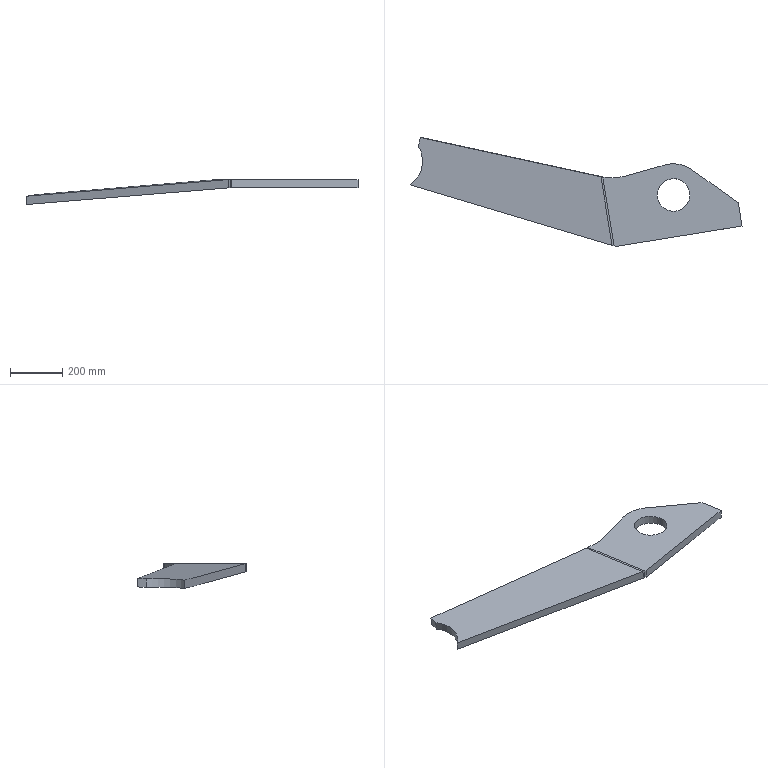Part | SolidWorks | features SplitBody 1 | 1 solid | 22 faces | box 1274 x 418.793 x 95.912 mm | volume 8572989 mm3 | plane 12 | cylinder 8 | spline 2 | commonest cylinder face diameters 125 x2 400 x2 100 x1 164 x1 220 x1 240 x1
STEP:
#1=CARTESIAN_POINT('',(4252.633,293.982,-770.5));
#2=VERTEX_POINT('',#1);
#3=CARTESIAN_POINT('',(4129.247,273.958,-770.5));
#4=VERTEX_POINT('',#3);
#5=CARTESIAN_POINT('',(4190.94,283.97,-770.5));
#6=DIRECTION('',(0.,0.,-1.));
#7=DIRECTION('',(-0.9871,-0.1602,0.));
#8=AXIS2_PLACEMENT_3D('',#5,#6,#7);
#9=CIRCLE('',#8,62.5);
#10=EDGE_CURVE('',#2,#4,#9,.T.);
#11=ORIENTED_EDGE('',*,*,#10,.F.);
#12=CARTESIAN_POINT('',(4252.633,293.982,-802.5));
#13=VERTEX_POINT('',#12);
#14=CARTESIAN_POINT('',(4252.633,293.982,-770.5));
#15=DIRECTION('',(0.,0.,-1.));
#16=VECTOR('',#15,1000.);
#17=LINE('',#14,#16);
#18=EDGE_CURVE('',#2,#13,#17,.T.);
#19=ORIENTED_EDGE('',*,*,#18,.T.);
#20=CARTESIAN_POINT('',(4129.247,273.958,-802.5));
#21=VERTEX_POINT('',#20);
#22=CARTESIAN_POINT('',(4190.94,283.97,-802.5));
#23=DIRECTION('',(0.,0.,-1.));
#24=DIRECTION('',(-0.9871,-0.1602,0.));
#25=AXIS2_PLACEMENT_3D('',#22,#23,#24);
#26=CIRCLE('',#25,62.5);
#27=EDGE_CURVE('',#13,#21,#26,.T.);
#28=ORIENTED_EDGE('',*,*,#27,.T.);
#29=CARTESIAN_POINT('',(4129.247,273.958,-770.5));
#30=DIRECTION('',(0.,0.,-1.));
#31=VECTOR('',#30,1000.);
#32=LINE('',#29,#31);
#33=EDGE_CURVE('',#4,#21,#32,.T.);
#34=ORIENTED_EDGE('',*,*,#33,.F.);
#35=EDGE_LOOP('',(#11,#19,#28,#34));
#36=FACE_OUTER_BOUND('',#35,.T.);
#37=CARTESIAN_POINT('',(4190.94,283.97,-770.5));
#38=DIRECTION('',(0.,0.,-1.));
#39=DIRECTION('',(-0.9871,-0.1602,0.));
#40=AXIS2_PLACEMENT_3D('',#37,#38,#39);
#41=CYLINDRICAL_SURFACE('',#40,62.5);
#42=ADVANCED_FACE('',(#36),#41,.F.);
#43=CARTESIAN_POINT('',(3957.472,90.301,-802.69));
#44=VERTEX_POINT('',#43);
#45=CARTESIAN_POINT('',(3914.616,354.364,-802.69));
#46=VERTEX_POINT('',#45);
#47=CARTESIAN_POINT('',(3884.78,538.207,-802.69));
#48=DIRECTION('',(-0.1602,0.9871,0.));
#49=VECTOR('',#48,1000.);
#50=LINE('',#47,#49);
#51=EDGE_CURVE('',#44,#46,#50,.T.);
#52=ORIENTED_EDGE('',*,*,#51,.F.);
#53=CARTESIAN_POINT('',(3181.855,322.901,-866.412));
#54=VERTEX_POINT('',#53);
#55=CARTESIAN_POINT('',(3181.855,322.901,-866.412));
#56=DIRECTION('',(0.9549,-0.2864,0.07845));
#57=VECTOR('',#56,1000.);
#58=LINE('',#55,#57);
#59=EDGE_CURVE('',#54,#44,#58,.T.);
#60=ORIENTED_EDGE('',*,*,#59,.F.);
#61=CARTESIAN_POINT('',(3214.351,471.062,-861.529));
#62=VERTEX_POINT('',#61);
#63=CARTESIAN_POINT('',(3120.615,414.189,-870.421));
#64=DIRECTION('',(0.08603,0.01396,-0.9962));
#65=DIRECTION('',(-0.9833,-0.1596,-0.08716));
#66=AXIS2_PLACEMENT_3D('',#63,#64,#65);
#67=CIRCLE('',#66,110.);
#68=EDGE_CURVE('',#62,#54,#67,.T.);
#69=ORIENTED_EDGE('',*,*,#68,.F.);
#70=CARTESIAN_POINT('',(3221.578,504.78,-860.432));
#71=VERTEX_POINT('',#70);
#72=CARTESIAN_POINT('',(3221.578,504.78,-860.432));
#73=DIRECTION('',(-0.2095,-0.9773,-0.03179));
#74=VECTOR('',#73,1000.);
#75=LINE('',#72,#74);
#76=EDGE_CURVE('',#71,#62,#75,.T.);
#77=ORIENTED_EDGE('',*,*,#76,.F.);
#78=CARTESIAN_POINT('',(3914.552,354.378,-802.696));
#79=VERTEX_POINT('',#78);
#80=CARTESIAN_POINT('',(3914.552,354.378,-802.696));
#81=DIRECTION('',(-0.974,0.2114,-0.08115));
#82=VECTOR('',#81,1000.);
#83=LINE('',#80,#82);
#84=EDGE_CURVE('',#79,#71,#83,.T.);
#85=ORIENTED_EDGE('',*,*,#84,.F.);
#86=CARTESIAN_POINT('',(3956.445,549.838,-796.338));
#87=DIRECTION('',(-0.08603,-0.01396,0.9962));
#88=DIRECTION('',(-0.9833,-0.1596,-0.08716));
#89=AXIS2_PLACEMENT_3D('',#86,#87,#88);
#90=CIRCLE('',#89,200.);
#91=EDGE_CURVE('',#79,#46,#90,.T.);
#92=ORIENTED_EDGE('',*,*,#91,.T.);
#93=EDGE_LOOP('',(#52,#60,#69,#77,#85,#92));
#94=FACE_OUTER_BOUND('',#93,.T.);
#95=CARTESIAN_POINT('',(3120.615,414.189,-870.421));
#96=DIRECTION('',(-0.08603,-0.01396,0.9962));
#97=DIRECTION('',(0.9833,0.1596,0.08716));
#98=AXIS2_PLACEMENT_3D('',#95,#96,#97);
#99=PLANE('',#98);
#100=ADVANCED_FACE('',(#94),#99,.F.);
#101=CARTESIAN_POINT('',(3919.263,352.938,-802.5));
#102=VERTEX_POINT('',#101);
#103=CARTESIAN_POINT('',(3919.263,352.938,-802.5));
#104=CARTESIAN_POINT('',(3917.712,353.413,-802.5));
#105=CARTESIAN_POINT('',(3916.162,353.888,-802.564));
#106=CARTESIAN_POINT('',(3914.616,354.364,-802.69));
#107=B_SPLINE_CURVE_WITH_KNOTS('',3,(#103,#104,#105,#106),.UNSPECIFIED.,.F.,.F.,(4,4),(0.,1.),.UNSPECIFIED.);
#108=EDGE_CURVE('',#102,#46,#107,.T.);
#109=ORIENTED_EDGE('',*,*,#108,.F.);
#110=CARTESIAN_POINT('',(3962.22,88.248,-802.5));
#111=VERTEX_POINT('',#110);
#112=CARTESIAN_POINT('',(3983.96,-45.707,-802.5));
#113=DIRECTION('',(-0.1602,0.9871,0.));
#114=VECTOR('',#113,1000.);
#115=LINE('',#112,#114);
#116=EDGE_CURVE('',#111,#102,#115,.T.);
#117=ORIENTED_EDGE('',*,*,#116,.F.);
#118=CARTESIAN_POINT('',(3957.472,90.301,-802.69));
#119=CARTESIAN_POINT('',(3959.051,89.616,-802.564));
#120=CARTESIAN_POINT('',(3960.635,88.932,-802.5));
#121=CARTESIAN_POINT('',(3962.22,88.248,-802.5));
#122=B_SPLINE_CURVE_WITH_KNOTS('',3,(#118,#119,#120,#121),.UNSPECIFIED.,.F.,.F.,(4,4),(0.,1.),.UNSPECIFIED.);
#123=EDGE_CURVE('',#44,#111,#122,.T.);
#124=ORIENTED_EDGE('',*,*,#123,.F.);
#125=ORIENTED_EDGE('',*,*,#51,.T.);
#126=EDGE_LOOP('',(#109,#117,#124,#125));
#127=FACE_OUTER_BOUND('',#126,.T.);
#128=CARTESIAN_POINT('',(3983.96,-45.707,-852.5));
#129=DIRECTION('',(-0.1602,0.9871,0.));
#130=DIRECTION('',(-0.08603,-0.01396,0.9962));
#131=AXIS2_PLACEMENT_3D('',#128,#129,#130);
#132=CYLINDRICAL_SURFACE('',#131,50.);
#133=ADVANCED_FACE('',(#127),#132,.F.);
#134=CARTESIAN_POINT('',(3954.719,89.855,-770.812));
#135=VERTEX_POINT('',#134);
#136=CARTESIAN_POINT('',(3954.719,89.855,-770.812));
#137=DIRECTION('',(0.08603,0.01396,-0.9962));
#138=VECTOR('',#137,1000.);
#139=LINE('',#136,#138);
#140=EDGE_CURVE('',#135,#44,#139,.T.);
#141=ORIENTED_EDGE('',*,*,#140,.F.);
#142=CARTESIAN_POINT('',(3179.102,322.454,-834.533));
#143=VERTEX_POINT('',#142);
#144=CARTESIAN_POINT('',(3179.102,322.454,-834.533));
#145=DIRECTION('',(0.9549,-0.2864,0.07845));
#146=VECTOR('',#145,1000.);
#147=LINE('',#144,#146);
#148=EDGE_CURVE('',#143,#135,#147,.T.);
#149=ORIENTED_EDGE('',*,*,#148,.F.);
#150=CARTESIAN_POINT('',(3179.102,322.454,-834.533));
#151=DIRECTION('',(-0.08603,-0.01396,0.9962));
#152=VECTOR('',#151,1000.);
#153=LINE('',#150,#152);
#154=EDGE_CURVE('',#54,#143,#153,.T.);
#155=ORIENTED_EDGE('',*,*,#154,.F.);
#156=ORIENTED_EDGE('',*,*,#59,.T.);
#157=EDGE_LOOP('',(#141,#149,#155,#156));
#158=FACE_OUTER_BOUND('',#157,.T.);
#159=CARTESIAN_POINT('',(3179.102,322.454,-834.533));
#160=DIRECTION('',(0.2842,0.958,0.03797));
#161=DIRECTION('',(-0.9549,0.2864,-0.07845));
#162=AXIS2_PLACEMENT_3D('',#159,#160,#161);
#163=PLANE('',#162);
#164=ADVANCED_FACE('',(#158),#163,.F.);
#165=ORIENTED_EDGE('',*,*,#154,.T.);
#166=CARTESIAN_POINT('',(3211.598,470.615,-829.651));
#167=VERTEX_POINT('',#166);
#168=CARTESIAN_POINT('',(3117.862,413.742,-838.543));
#169=DIRECTION('',(0.08603,0.01396,-0.9962));
#170=DIRECTION('',(-0.9833,-0.1596,-0.08716));
#171=AXIS2_PLACEMENT_3D('',#168,#169,#170);
#172=CIRCLE('',#171,110.);
#173=EDGE_CURVE('',#167,#143,#172,.T.);
#174=ORIENTED_EDGE('',*,*,#173,.F.);
#175=CARTESIAN_POINT('',(3211.598,470.615,-829.651));
#176=DIRECTION('',(-0.08603,-0.01396,0.9962));
#177=VECTOR('',#176,1000.);
#178=LINE('',#175,#177);
#179=EDGE_CURVE('',#62,#167,#178,.T.);
#180=ORIENTED_EDGE('',*,*,#179,.F.);
#181=ORIENTED_EDGE('',*,*,#68,.T.);
#182=EDGE_LOOP('',(#165,#174,#180,#181));
#183=FACE_OUTER_BOUND('',#182,.T.);
#184=CARTESIAN_POINT('',(3117.862,413.742,-838.543));
#185=DIRECTION('',(0.08603,0.01396,-0.9962));
#186=DIRECTION('',(-0.9833,-0.1596,-0.08716));
#187=AXIS2_PLACEMENT_3D('',#184,#185,#186);
#188=CYLINDRICAL_SURFACE('',#187,110.);
#189=ADVANCED_FACE('',(#183),#188,.F.);
#190=ORIENTED_EDGE('',*,*,#179,.T.);
#191=CARTESIAN_POINT('',(3218.825,504.333,-828.554));
#192=VERTEX_POINT('',#191);
#193=CARTESIAN_POINT('',(3218.825,504.333,-828.554));
#194=DIRECTION('',(-0.2095,-0.9773,-0.03179));
#195=VECTOR('',#194,1000.);
#196=LINE('',#193,#195);
#197=EDGE_CURVE('',#192,#167,#196,.T.);
#198=ORIENTED_EDGE('',*,*,#197,.F.);
#199=CARTESIAN_POINT('',(3218.825,504.333,-828.554));
#200=DIRECTION('',(-0.08603,-0.01396,0.9962));
#201=VECTOR('',#200,1000.);
#202=LINE('',#199,#201);
#203=EDGE_CURVE('',#71,#192,#202,.T.);
#204=ORIENTED_EDGE('',*,*,#203,.F.);
#205=ORIENTED_EDGE('',*,*,#76,.T.);
#206=EDGE_LOOP('',(#190,#198,#204,#205));
#207=FACE_OUTER_BOUND('',#206,.T.);
#208=CARTESIAN_POINT('',(3218.825,504.333,-828.554));
#209=DIRECTION('',(0.974,-0.2114,0.08115));
#210=DIRECTION('',(0.2095,0.9773,0.03179));
#211=AXIS2_PLACEMENT_3D('',#208,#209,#210);
#212=PLANE('',#211);
#213=ADVANCED_FACE('',(#207),#212,.F.);
#214=ORIENTED_EDGE('',*,*,#203,.T.);
#215=CARTESIAN_POINT('',(3911.799,353.931,-770.817));
#216=VERTEX_POINT('',#215);
#217=CARTESIAN_POINT('',(3218.825,504.333,-828.554));
#218=DIRECTION('',(-0.974,0.2114,-0.08115));
#219=VECTOR('',#218,1000.);
#220=LINE('',#217,#219);
#221=EDGE_CURVE('',#216,#192,#220,.T.);
#222=ORIENTED_EDGE('',*,*,#221,.F.);
#223=CARTESIAN_POINT('',(3911.799,353.931,-770.817));
#224=DIRECTION('',(-0.08603,-0.01396,0.9962));
#225=VECTOR('',#224,1000.);
#226=LINE('',#223,#225);
#227=EDGE_CURVE('',#79,#216,#226,.T.);
#228=ORIENTED_EDGE('',*,*,#227,.F.);
#229=ORIENTED_EDGE('',*,*,#84,.T.);
#230=EDGE_LOOP('',(#214,#222,#228,#229));
#231=FACE_OUTER_BOUND('',#230,.T.);
#232=CARTESIAN_POINT('',(3218.825,504.333,-828.554));
#233=DIRECTION('',(-0.2095,-0.9773,-0.03179));
#234=DIRECTION('',(0.974,-0.2114,0.08115));
#235=AXIS2_PLACEMENT_3D('',#232,#233,#234);
#236=PLANE('',#235);
#237=ADVANCED_FACE('',(#231),#236,.F.);
#238=CARTESIAN_POINT('',(3911.863,353.917,-770.812));
#239=VERTEX_POINT('',#238);
#240=CARTESIAN_POINT('',(3913.24,354.141,-786.751));
#241=DIRECTION('',(-0.08603,-0.01396,0.9962));
#242=VECTOR('',#241,1000.);
#243=LINE('',#240,#242);
#244=EDGE_CURVE('',#46,#239,#243,.T.);
#245=ORIENTED_EDGE('',*,*,#244,.T.);
#246=CARTESIAN_POINT('',(3919.263,352.938,-770.5));
#247=VERTEX_POINT('',#246);
#248=CARTESIAN_POINT('',(3911.863,353.917,-770.812));
#249=CARTESIAN_POINT('',(3914.324,353.59,-770.604));
#250=CARTESIAN_POINT('',(3916.793,353.264,-770.5));
#251=CARTESIAN_POINT('',(3919.263,352.938,-770.5));
#252=B_SPLINE_CURVE_WITH_KNOTS('',3,(#248,#249,#250,#251),.UNSPECIFIED.,.F.,.F.,(4,4),(0.,1.),.UNSPECIFIED.);
#253=EDGE_CURVE('',#239,#247,#252,.T.);
#254=ORIENTED_EDGE('',*,*,#253,.T.);
#255=CARTESIAN_POINT('',(3919.263,352.938,-786.5));
#256=DIRECTION('',(0.,0.,-1.));
#257=VECTOR('',#256,1000.);
#258=LINE('',#255,#257);
#259=EDGE_CURVE('',#247,#102,#258,.T.);
#260=ORIENTED_EDGE('',*,*,#259,.T.);
#261=ORIENTED_EDGE('',*,*,#108,.T.);
#262=EDGE_LOOP('',(#245,#254,#260,#261));
#263=FACE_OUTER_BOUND('',#262,.T.);
#264=CARTESIAN_POINT('',(3919.263,352.938,-770.18));
#265=CARTESIAN_POINT('',(3916.784,353.262,-770.18));
#266=CARTESIAN_POINT('',(3914.306,353.587,-770.285));
#267=CARTESIAN_POINT('',(3911.836,353.913,-770.493));
#268=CARTESIAN_POINT('',(3919.263,352.938,-770.5));
#269=CARTESIAN_POINT('',(3916.793,353.264,-770.5));
#270=CARTESIAN_POINT('',(3914.324,353.59,-770.604));
#271=CARTESIAN_POINT('',(3911.863,353.917,-770.812));
#272=CARTESIAN_POINT('',(3919.263,352.938,-802.5));
#273=CARTESIAN_POINT('',(3917.712,353.413,-802.5));
#274=CARTESIAN_POINT('',(3916.162,353.888,-802.564));
#275=CARTESIAN_POINT('',(3914.616,354.364,-802.69));
#276=B_SPLINE_SURFACE_WITH_KNOTS('',1,3,((#264,#265,#266,#267),(#268,#269,#270,#271),(#272,#273,#274,#275)),.UNSPECIFIED.,.F.,.F.,.F.,(2,1,2),(4,4),(-0.01,0.,1.),(0.,1.),.UNSPECIFIED.);
#277=ADVANCED_FACE('',(#263),#276,.T.);
#278=CARTESIAN_POINT('',(4190.94,283.97,-802.5));
#279=DIRECTION('',(0.,0.,-1.));
#280=DIRECTION('',(-0.9871,-0.1602,0.));
#281=AXIS2_PLACEMENT_3D('',#278,#279,#280);
#282=CIRCLE('',#281,62.5);
#283=EDGE_CURVE('',#21,#13,#282,.T.);
#284=ORIENTED_EDGE('',*,*,#283,.F.);
#285=ORIENTED_EDGE('',*,*,#27,.F.);
#286=EDGE_LOOP('',(#284,#285));
#287=FACE_BOUND('',#286,.T.);
#288=CARTESIAN_POINT('',(4010.04,357.285,-802.5));
#289=VERTEX_POINT('',#288);
#290=CARTESIAN_POINT('',(3955.335,549.658,-802.5));
#291=DIRECTION('',(0.,0.,-1.));
#292=DIRECTION('',(-0.9871,-0.1602,0.));
#293=AXIS2_PLACEMENT_3D('',#290,#291,#292);
#294=CIRCLE('',#293,200.);
#295=EDGE_CURVE('',#289,#102,#294,.T.);
#296=ORIENTED_EDGE('',*,*,#295,.F.);
#297=CARTESIAN_POINT('',(4158.117,399.394,-802.5));
#298=VERTEX_POINT('',#297);
#299=CARTESIAN_POINT('',(4158.117,399.394,-802.5));
#300=DIRECTION('',(-0.9619,-0.2735,0.));
#301=VECTOR('',#300,1000.);
#302=LINE('',#299,#301);
#303=EDGE_CURVE('',#298,#289,#302,.T.);
#304=ORIENTED_EDGE('',*,*,#303,.F.);
#305=CARTESIAN_POINT('',(4261.011,381.386,-802.5));
#306=VERTEX_POINT('',#305);
#307=CARTESIAN_POINT('',(4190.94,283.97,-802.5));
#308=DIRECTION('',(0.,0.,1.));
#309=DIRECTION('',(-0.9871,-0.1602,0.));
#310=AXIS2_PLACEMENT_3D('',#307,#308,#309);
#311=CIRCLE('',#310,120.);
#312=EDGE_CURVE('',#306,#298,#311,.T.);
#313=ORIENTED_EDGE('',*,*,#312,.F.);
#314=CARTESIAN_POINT('',(4439.054,253.321,-802.5));
#315=VERTEX_POINT('',#314);
#316=CARTESIAN_POINT('',(4439.054,253.321,-802.5));
#317=DIRECTION('',(-0.8118,0.5839,0.));
#318=VECTOR('',#317,1000.);
#319=LINE('',#316,#318);
#320=EDGE_CURVE('',#315,#306,#319,.T.);
#321=ORIENTED_EDGE('',*,*,#320,.F.);
#322=CARTESIAN_POINT('',(4453.472,164.483,-802.5));
#323=VERTEX_POINT('',#322);
#324=CARTESIAN_POINT('',(4379.781,618.543,-802.5));
#325=DIRECTION('',(-0.1602,0.9871,0.));
#326=VECTOR('',#325,1000.);
#327=LINE('',#324,#326);
#328=EDGE_CURVE('',#323,#315,#327,.T.);
#329=ORIENTED_EDGE('',*,*,#328,.F.);
#330=CARTESIAN_POINT('',(3969.8,85.987,-802.5));
#331=VERTEX_POINT('',#330);
#332=CARTESIAN_POINT('',(3190.003,-40.568,-802.5));
#333=DIRECTION('',(0.9871,0.1602,0.));
#334=VECTOR('',#333,1000.);
#335=LINE('',#332,#334);
#336=EDGE_CURVE('',#331,#323,#335,.T.);
#337=ORIENTED_EDGE('',*,*,#336,.F.);
#338=CARTESIAN_POINT('',(3962.22,88.248,-802.5));
#339=DIRECTION('',(0.9583,-0.2858,0.));
#340=VECTOR('',#339,1000.);
#341=LINE('',#338,#340);
#342=EDGE_CURVE('',#111,#331,#341,.T.);
#343=ORIENTED_EDGE('',*,*,#342,.F.);
#344=ORIENTED_EDGE('',*,*,#116,.T.);
#345=EDGE_LOOP('',(#296,#304,#313,#321,#329,#337,#343,#344));
#346=FACE_OUTER_BOUND('',#345,.T.);
#347=CARTESIAN_POINT('',(3116.313,413.491,-802.5));
#348=DIRECTION('',(0.,0.,1.));
#349=DIRECTION('',(0.9871,0.1602,0.));
#350=AXIS2_PLACEMENT_3D('',#347,#348,#349);
#351=PLANE('',#350);
#352=ADVANCED_FACE('',(#287,#346),#351,.F.);
#353=CARTESIAN_POINT('',(3962.22,88.248,-770.5));
#354=VERTEX_POINT('',#353);
#355=CARTESIAN_POINT('',(3962.22,88.248,-770.5));
#356=CARTESIAN_POINT('',(3959.717,88.783,-770.5));
#357=CARTESIAN_POINT('',(3957.213,89.318,-770.604));
#358=CARTESIAN_POINT('',(3954.719,89.855,-770.812));
#359=B_SPLINE_CURVE_WITH_KNOTS('',3,(#355,#356,#357,#358),.UNSPECIFIED.,.F.,.F.,(4,4),(0.,1.),.UNSPECIFIED.);
#360=EDGE_CURVE('',#354,#135,#359,.T.);
#361=ORIENTED_EDGE('',*,*,#360,.T.);
#362=ORIENTED_EDGE('',*,*,#140,.T.);
#363=ORIENTED_EDGE('',*,*,#123,.T.);
#364=CARTESIAN_POINT('',(3962.22,88.248,-786.5));
#365=DIRECTION('',(0.,0.,1.));
#366=VECTOR('',#365,1000.);
#367=LINE('',#364,#366);
#368=EDGE_CURVE('',#111,#354,#367,.T.);
#369=ORIENTED_EDGE('',*,*,#368,.T.);
#370=EDGE_LOOP('',(#361,#362,#363,#369));
#371=FACE_OUTER_BOUND('',#370,.T.);
#372=CARTESIAN_POINT('',(3954.691,89.85,-770.493));
#373=CARTESIAN_POINT('',(3957.195,89.315,-770.285));
#374=CARTESIAN_POINT('',(3959.707,88.782,-770.18));
#375=CARTESIAN_POINT('',(3962.22,88.248,-770.18));
#376=CARTESIAN_POINT('',(3954.719,89.855,-770.812));
#377=CARTESIAN_POINT('',(3957.213,89.318,-770.604));
#378=CARTESIAN_POINT('',(3959.717,88.783,-770.5));
#379=CARTESIAN_POINT('',(3962.22,88.248,-770.5));
#380=CARTESIAN_POINT('',(3957.472,90.301,-802.69));
#381=CARTESIAN_POINT('',(3959.051,89.616,-802.564));
#382=CARTESIAN_POINT('',(3960.635,88.932,-802.5));
#383=CARTESIAN_POINT('',(3962.22,88.248,-802.5));
#384=B_SPLINE_SURFACE_WITH_KNOTS('',1,3,((#372,#373,#374,#375),(#376,#377,#378,#379),(#380,#381,#382,#383)),.UNSPECIFIED.,.F.,.F.,.F.,(2,1,2),(4,4),(-0.01,0.,1.),(0.,1.),.UNSPECIFIED.);
#385=ADVANCED_FACE('',(#371),#384,.T.);
#386=ORIENTED_EDGE('',*,*,#173,.T.);
#387=ORIENTED_EDGE('',*,*,#148,.T.);
#388=CARTESIAN_POINT('',(3882.027,537.761,-770.812));
#389=DIRECTION('',(-0.1602,0.9871,0.));
#390=VECTOR('',#389,1000.);
#391=LINE('',#388,#390);
#392=EDGE_CURVE('',#135,#239,#391,.T.);
#393=ORIENTED_EDGE('',*,*,#392,.T.);
#394=CARTESIAN_POINT('',(3911.863,353.917,-770.812));
#395=DIRECTION('',(-0.9741,0.2112,-0.08116));
#396=VECTOR('',#395,1000.);
#397=LINE('',#394,#396);
#398=EDGE_CURVE('',#239,#216,#397,.T.);
#399=ORIENTED_EDGE('',*,*,#398,.T.);
#400=ORIENTED_EDGE('',*,*,#221,.T.);
#401=ORIENTED_EDGE('',*,*,#197,.T.);
#402=EDGE_LOOP('',(#386,#387,#393,#399,#400,#401));
#403=FACE_OUTER_BOUND('',#402,.T.);
#404=CARTESIAN_POINT('',(3117.862,413.742,-838.543));
#405=DIRECTION('',(-0.08603,-0.01396,0.9962));
#406=DIRECTION('',(0.9833,0.1596,0.08716));
#407=AXIS2_PLACEMENT_3D('',#404,#405,#406);
#408=PLANE('',#407);
#409=ADVANCED_FACE('',(#403),#408,.T.);
#410=ORIENTED_EDGE('',*,*,#244,.F.);
#411=ORIENTED_EDGE('',*,*,#91,.F.);
#412=ORIENTED_EDGE('',*,*,#227,.T.);
#413=ORIENTED_EDGE('',*,*,#398,.F.);
#414=EDGE_LOOP('',(#410,#411,#412,#413));
#415=FACE_OUTER_BOUND('',#414,.T.);
#416=CARTESIAN_POINT('',(3953.692,549.391,-764.46));
#417=DIRECTION('',(0.08603,0.01396,-0.9962));
#418=DIRECTION('',(-0.9833,-0.1596,-0.08716));
#419=AXIS2_PLACEMENT_3D('',#416,#417,#418);
#420=CYLINDRICAL_SURFACE('',#419,200.);
#421=ADVANCED_FACE('',(#415),#420,.F.);
#422=CARTESIAN_POINT('',(3983.96,-45.707,-770.5));
#423=DIRECTION('',(-0.1602,0.9871,0.));
#424=VECTOR('',#423,1000.);
#425=LINE('',#422,#424);
#426=EDGE_CURVE('',#354,#247,#425,.T.);
#427=ORIENTED_EDGE('',*,*,#426,.T.);
#428=ORIENTED_EDGE('',*,*,#253,.F.);
#429=ORIENTED_EDGE('',*,*,#392,.F.);
#430=ORIENTED_EDGE('',*,*,#360,.F.);
#431=EDGE_LOOP('',(#427,#428,#429,#430));
#432=FACE_OUTER_BOUND('',#431,.T.);
#433=CARTESIAN_POINT('',(3983.96,-45.707,-852.5));
#434=DIRECTION('',(-0.1602,0.9871,0.));
#435=DIRECTION('',(-0.08603,-0.01396,0.9962));
#436=AXIS2_PLACEMENT_3D('',#433,#434,#435);
#437=CYLINDRICAL_SURFACE('',#436,82.);
#438=ADVANCED_FACE('',(#432),#437,.T.);
#439=CARTESIAN_POINT('',(4010.04,357.285,-770.5));
#440=VERTEX_POINT('',#439);
#441=CARTESIAN_POINT('',(3955.335,549.658,-770.5));
#442=DIRECTION('',(0.,0.,-1.));
#443=DIRECTION('',(-0.9871,-0.1602,0.));
#444=AXIS2_PLACEMENT_3D('',#441,#442,#443);
#445=CIRCLE('',#444,200.);
#446=EDGE_CURVE('',#440,#247,#445,.T.);
#447=ORIENTED_EDGE('',*,*,#446,.F.);
#448=CARTESIAN_POINT('',(4010.04,357.285,-770.5));
#449=DIRECTION('',(0.,0.,1.));
#450=VECTOR('',#449,1000.);
#451=LINE('',#448,#450);
#452=EDGE_CURVE('',#289,#440,#451,.T.);
#453=ORIENTED_EDGE('',*,*,#452,.F.);
#454=ORIENTED_EDGE('',*,*,#295,.T.);
#455=ORIENTED_EDGE('',*,*,#259,.F.);
#456=EDGE_LOOP('',(#447,#453,#454,#455));
#457=FACE_OUTER_BOUND('',#456,.T.);
#458=CARTESIAN_POINT('',(3955.335,549.658,-770.5));
#459=DIRECTION('',(0.,0.,-1.));
#460=DIRECTION('',(-0.9871,-0.1602,0.));
#461=AXIS2_PLACEMENT_3D('',#458,#459,#460);
#462=CYLINDRICAL_SURFACE('',#461,200.);
#463=ADVANCED_FACE('',(#457),#462,.F.);
#464=ORIENTED_EDGE('',*,*,#18,.F.);
#465=CARTESIAN_POINT('',(4190.94,283.97,-770.5));
#466=DIRECTION('',(0.,0.,-1.));
#467=DIRECTION('',(-0.9871,-0.1602,0.));
#468=AXIS2_PLACEMENT_3D('',#465,#466,#467);
#469=CIRCLE('',#468,62.5);
#470=EDGE_CURVE('',#4,#2,#469,.T.);
#471=ORIENTED_EDGE('',*,*,#470,.F.);
#472=ORIENTED_EDGE('',*,*,#33,.T.);
#473=ORIENTED_EDGE('',*,*,#283,.T.);
#474=EDGE_LOOP('',(#464,#471,#472,#473));
#475=FACE_OUTER_BOUND('',#474,.T.);
#476=CARTESIAN_POINT('',(4190.94,283.97,-770.5));
#477=DIRECTION('',(0.,0.,-1.));
#478=DIRECTION('',(-0.9871,-0.1602,0.));
#479=AXIS2_PLACEMENT_3D('',#476,#477,#478);
#480=CYLINDRICAL_SURFACE('',#479,62.5);
#481=ADVANCED_FACE('',(#475),#480,.F.);
#482=ORIENTED_EDGE('',*,*,#452,.T.);
#483=CARTESIAN_POINT('',(4158.117,399.394,-770.5));
#484=VERTEX_POINT('',#483);
#485=CARTESIAN_POINT('',(4158.117,399.394,-770.5));
#486=DIRECTION('',(-0.9619,-0.2735,0.));
#487=VECTOR('',#486,1000.);
#488=LINE('',#485,#487);
#489=EDGE_CURVE('',#484,#440,#488,.T.);
#490=ORIENTED_EDGE('',*,*,#489,.F.);
#491=CARTESIAN_POINT('',(4158.117,399.394,-802.5));
#492=DIRECTION('',(0.,0.,1.));
#493=VECTOR('',#492,1000.);
#494=LINE('',#491,#493);
#495=EDGE_CURVE('',#298,#484,#494,.T.);
#496=ORIENTED_EDGE('',*,*,#495,.F.);
#497=ORIENTED_EDGE('',*,*,#303,.T.);
#498=EDGE_LOOP('',(#482,#490,#496,#497));
#499=FACE_OUTER_BOUND('',#498,.T.);
#500=CARTESIAN_POINT('',(4158.117,399.394,-770.5));
#501=DIRECTION('',(0.2735,-0.9619,0.));
#502=DIRECTION('',(0.9583,0.2725,0.08657));
#503=AXIS2_PLACEMENT_3D('',#500,#501,#502);
#504=PLANE('',#503);
#505=ADVANCED_FACE('',(#499),#504,.F.);
#506=CARTESIAN_POINT('',(4261.011,381.386,-770.5));
#507=VERTEX_POINT('',#506);
#508=CARTESIAN_POINT('',(4190.94,283.97,-770.5));
#509=DIRECTION('',(0.,0.,-1.));
#510=DIRECTION('',(-0.9871,-0.1602,0.));
#511=AXIS2_PLACEMENT_3D('',#508,#509,#510);
#512=CIRCLE('',#511,120.);
#513=EDGE_CURVE('',#484,#507,#512,.T.);
#514=ORIENTED_EDGE('',*,*,#513,.T.);
#515=CARTESIAN_POINT('',(4261.011,381.386,-770.5));
#516=DIRECTION('',(0.,0.,-1.));
#517=VECTOR('',#516,1000.);
#518=LINE('',#515,#517);
#519=EDGE_CURVE('',#507,#306,#518,.T.);
#520=ORIENTED_EDGE('',*,*,#519,.T.);
#521=ORIENTED_EDGE('',*,*,#312,.T.);
#522=ORIENTED_EDGE('',*,*,#495,.T.);
#523=EDGE_LOOP('',(#514,#520,#521,#522));
#524=FACE_OUTER_BOUND('',#523,.T.);
#525=CARTESIAN_POINT('',(4190.94,283.97,-770.5));
#526=DIRECTION('',(0.,0.,-1.));
#527=DIRECTION('',(-0.9871,-0.1602,0.));
#528=AXIS2_PLACEMENT_3D('',#525,#526,#527);
#529=CYLINDRICAL_SURFACE('',#528,120.);
#530=ADVANCED_FACE('',(#524),#529,.T.);
#531=ORIENTED_EDGE('',*,*,#519,.F.);
#532=CARTESIAN_POINT('',(4439.054,253.321,-770.5));
#533=VERTEX_POINT('',#532);
#534=CARTESIAN_POINT('',(4439.054,253.321,-770.5));
#535=DIRECTION('',(-0.8118,0.5839,0.));
#536=VECTOR('',#535,1000.);
#537=LINE('',#534,#536);
#538=EDGE_CURVE('',#533,#507,#537,.T.);
#539=ORIENTED_EDGE('',*,*,#538,.F.);
#540=CARTESIAN_POINT('',(4439.054,253.321,-802.5));
#541=DIRECTION('',(0.,0.,1.));
#542=VECTOR('',#541,1000.);
#543=LINE('',#540,#542);
#544=EDGE_CURVE('',#315,#533,#543,.T.);
#545=ORIENTED_EDGE('',*,*,#544,.F.);
#546=ORIENTED_EDGE('',*,*,#320,.T.);
#547=EDGE_LOOP('',(#531,#539,#545,#546));
#548=FACE_OUTER_BOUND('',#547,.T.);
#549=CARTESIAN_POINT('',(4439.054,253.321,-770.5));
#550=DIRECTION('',(-0.5839,-0.8118,0.));
#551=DIRECTION('',(0.8103,-0.5828,0.0618));
#552=AXIS2_PLACEMENT_3D('',#549,#550,#551);
#553=PLANE('',#552);
#554=ADVANCED_FACE('',(#548),#553,.F.);
#555=ORIENTED_EDGE('',*,*,#544,.T.);
#556=CARTESIAN_POINT('',(4453.472,164.483,-770.5));
#557=VERTEX_POINT('',#556);
#558=CARTESIAN_POINT('',(4453.472,164.483,-770.5));
#559=DIRECTION('',(-0.1602,0.9871,0.));
#560=VECTOR('',#559,1000.);
#561=LINE('',#558,#560);
#562=EDGE_CURVE('',#557,#533,#561,.T.);
#563=ORIENTED_EDGE('',*,*,#562,.F.);
#564=CARTESIAN_POINT('',(4453.472,164.483,-770.5));
#565=DIRECTION('',(0.,0.,1.));
#566=VECTOR('',#565,1000.);
#567=LINE('',#564,#566);
#568=EDGE_CURVE('',#323,#557,#567,.T.);
#569=ORIENTED_EDGE('',*,*,#568,.F.);
#570=ORIENTED_EDGE('',*,*,#328,.T.);
#571=EDGE_LOOP('',(#555,#563,#569,#570));
#572=FACE_OUTER_BOUND('',#571,.T.);
#573=CARTESIAN_POINT('',(4453.472,164.483,-770.5));
#574=DIRECTION('',(-0.9871,-0.1602,0.));
#575=DIRECTION('',(0.,0.,1.));
#576=AXIS2_PLACEMENT_3D('',#573,#574,#575);
#577=PLANE('',#576);
#578=ADVANCED_FACE('',(#572),#577,.F.);
#579=ORIENTED_EDGE('',*,*,#568,.T.);
#580=CARTESIAN_POINT('',(3969.8,85.987,-770.5));
#581=VERTEX_POINT('',#580);
#582=CARTESIAN_POINT('',(3969.8,85.987,-770.5));
#583=DIRECTION('',(0.9871,0.1602,0.));
#584=VECTOR('',#583,1000.);
#585=LINE('',#582,#584);
#586=EDGE_CURVE('',#581,#557,#585,.T.);
#587=ORIENTED_EDGE('',*,*,#586,.F.);
#588=CARTESIAN_POINT('',(3969.8,85.987,-802.5));
#589=DIRECTION('',(0.,0.,1.));
#590=VECTOR('',#589,1000.);
#591=LINE('',#588,#590);
#592=EDGE_CURVE('',#331,#581,#591,.T.);
#593=ORIENTED_EDGE('',*,*,#592,.F.);
#594=ORIENTED_EDGE('',*,*,#336,.T.);
#595=EDGE_LOOP('',(#579,#587,#593,#594));
#596=FACE_OUTER_BOUND('',#595,.T.);
#597=CARTESIAN_POINT('',(3969.8,85.987,-770.5));
#598=DIRECTION('',(-0.1602,0.9871,0.));
#599=DIRECTION('',(-0.08603,-0.01396,0.9962));
#600=AXIS2_PLACEMENT_3D('',#597,#598,#599);
#601=PLANE('',#600);
#602=ADVANCED_FACE('',(#596),#601,.F.);
#603=ORIENTED_EDGE('',*,*,#342,.T.);
#604=ORIENTED_EDGE('',*,*,#592,.T.);
#605=CARTESIAN_POINT('',(3962.22,88.248,-770.5));
#606=DIRECTION('',(0.9583,-0.2858,0.));
#607=VECTOR('',#606,1000.);
#608=LINE('',#605,#607);
#609=EDGE_CURVE('',#354,#581,#608,.T.);
#610=ORIENTED_EDGE('',*,*,#609,.F.);
#611=ORIENTED_EDGE('',*,*,#368,.F.);
#612=EDGE_LOOP('',(#603,#604,#610,#611));
#613=FACE_OUTER_BOUND('',#612,.T.);
#614=CARTESIAN_POINT('',(3177.725,322.23,-770.5));
#615=DIRECTION('',(0.2858,0.9583,0.));
#616=DIRECTION('',(-0.9553,0.2849,-0.07851));
#617=AXIS2_PLACEMENT_3D('',#614,#615,#616);
#618=PLANE('',#617);
#619=ADVANCED_FACE('',(#613),#618,.F.);
#620=ORIENTED_EDGE('',*,*,#513,.F.);
#621=ORIENTED_EDGE('',*,*,#489,.T.);
#622=ORIENTED_EDGE('',*,*,#446,.T.);
#623=ORIENTED_EDGE('',*,*,#426,.F.);
#624=ORIENTED_EDGE('',*,*,#609,.T.);
#625=ORIENTED_EDGE('',*,*,#586,.T.);
#626=ORIENTED_EDGE('',*,*,#562,.T.);
#627=ORIENTED_EDGE('',*,*,#538,.T.);
#628=EDGE_LOOP('',(#620,#621,#622,#623,#624,#625,#626,#627));
#629=FACE_OUTER_BOUND('',#628,.T.);
#630=ORIENTED_EDGE('',*,*,#470,.T.);
#631=ORIENTED_EDGE('',*,*,#10,.T.);
#632=EDGE_LOOP('',(#630,#631));
#633=FACE_BOUND('',#632,.T.);
#634=CARTESIAN_POINT('',(3116.313,413.491,-770.5));
#635=DIRECTION('',(0.,0.,1.));
#636=DIRECTION('',(0.9871,0.1602,0.));
#637=AXIS2_PLACEMENT_3D('',#634,#635,#636);
#638=PLANE('',#637);
#639=ADVANCED_FACE('',(#629,#633),#638,.T.);
#640=CLOSED_SHELL('',(#42,#100,#133,#164,#189,#213,#237,#277,#352,#385,#409,#421,#438,#463,#481,#505,#530,#554,#578,#602,#619,#639));
#641=MANIFOLD_SOLID_BREP('',#640);
#642=CARTESIAN_POINT('',(0.,0.,0.));
#643=DIRECTION('',(0.,0.,1.));
#644=DIRECTION('',(1.,0.,0.));
#645=AXIS2_PLACEMENT_3D('',#642,#643,#644);
#646=(LENGTH_UNIT()NAMED_UNIT(*)SI_UNIT(.MILLI.,.METRE.));
#647=UNCERTAINTY_MEASURE_WITH_UNIT(LENGTH_MEASURE(0.00001),#646,'','');
#648=(NAMED_UNIT(*)PLANE_ANGLE_UNIT()SI_UNIT($,.RADIAN.));
#649=(NAMED_UNIT(*)SI_UNIT($,.STERADIAN.)SOLID_ANGLE_UNIT());
#650=(GEOMETRIC_REPRESENTATION_CONTEXT(3)GLOBAL_UNCERTAINTY_ASSIGNED_CONTEXT((#647))GLOBAL_UNIT_ASSIGNED_CONTEXT((#646,#648,#649))REPRESENTATION_CONTEXT('',''));
#651=ADVANCED_BREP_SHAPE_REPRESENTATION('',(#641,#645),#650);